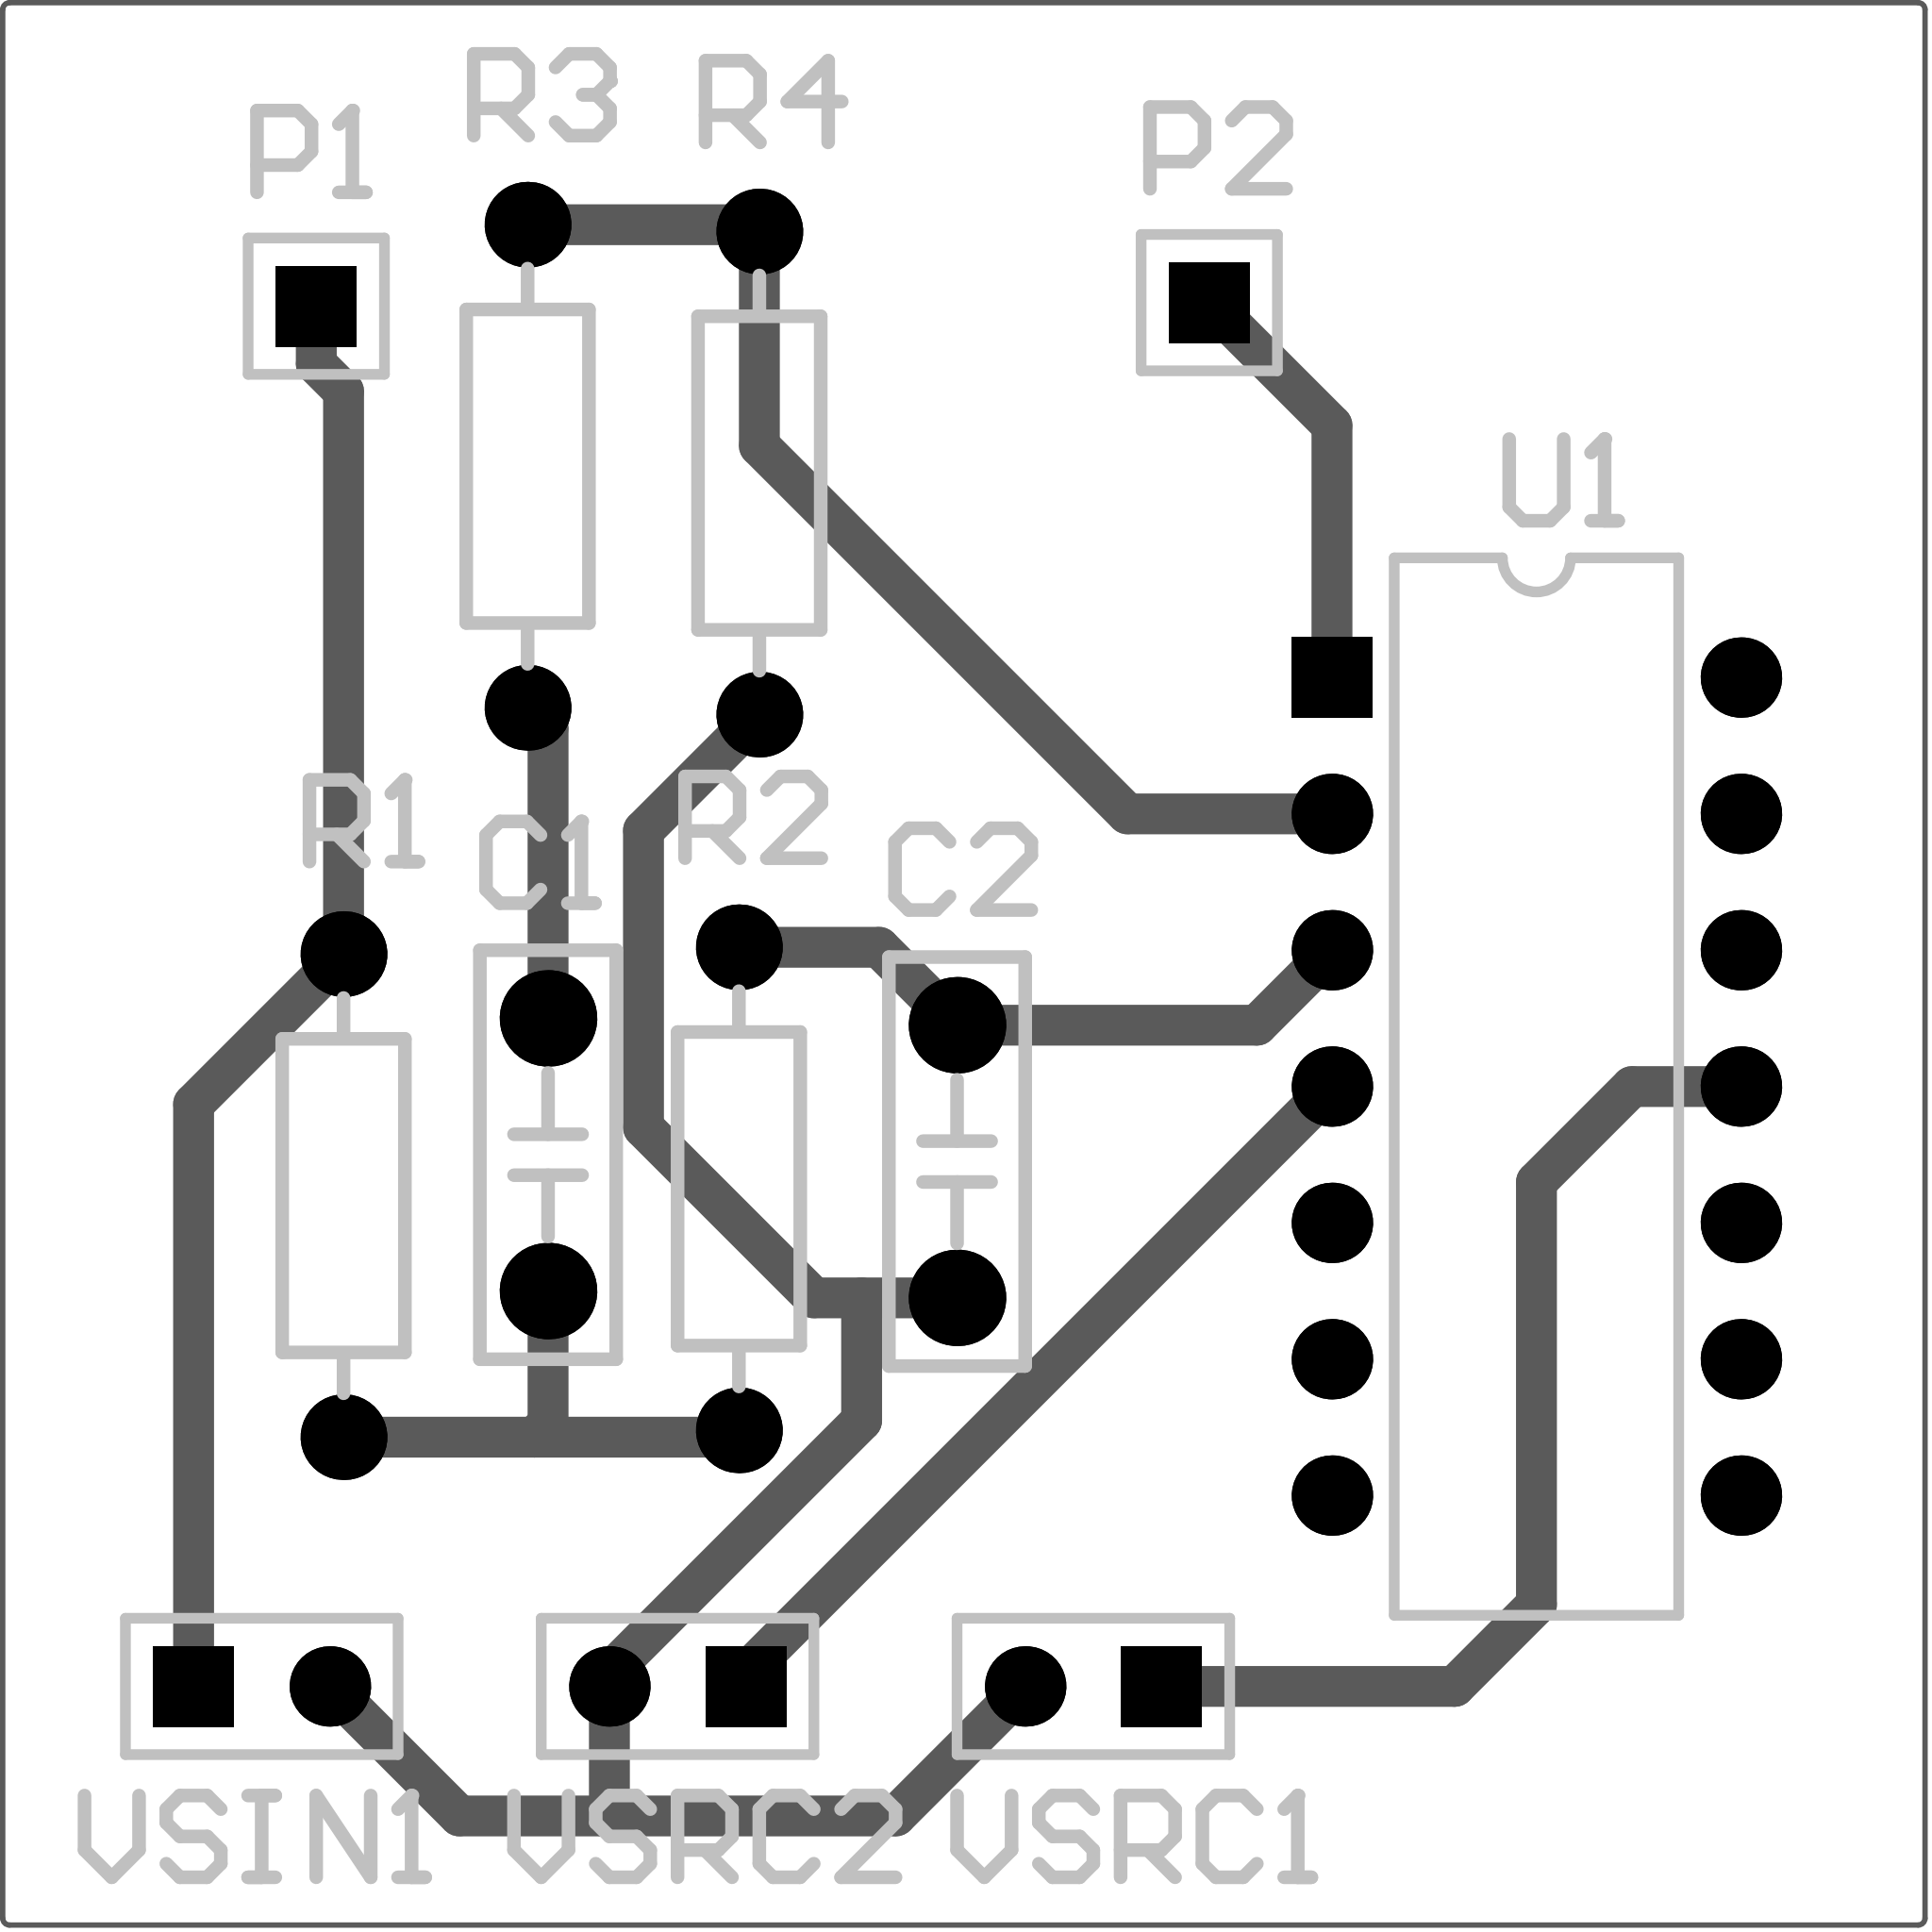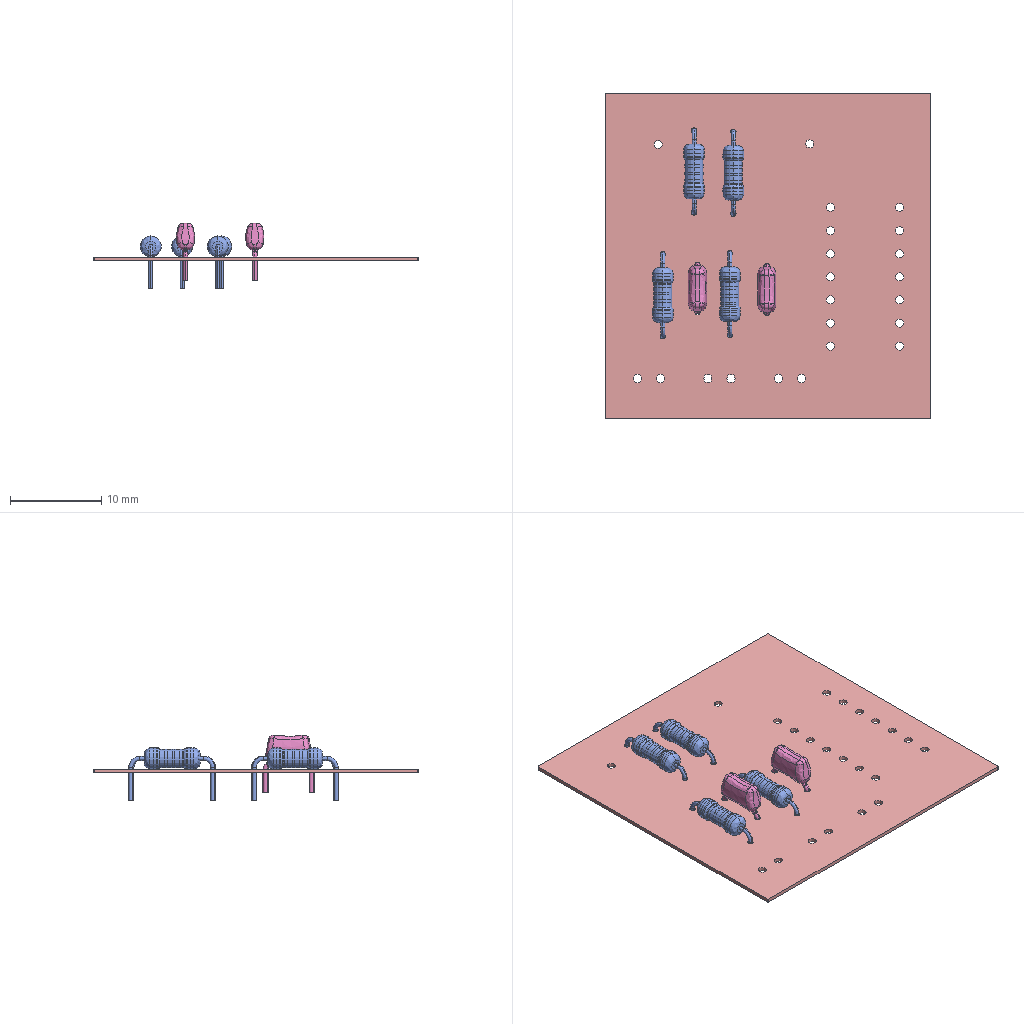Circuit board layout | Altium Designer | box 35.8 x 35.8 x 7.2 mm
Layer stack:
# Altium Designer layer stack of  (unit mm; dielectric type: 0 none, 1 core, 2 prepreg, 3 surface material)
index,name,kind,layer,copper_thickness_mm,dielectric_type,dielectric_thickness_mm,dielectric_material,dielectric_constant
0,Top Paste,other,,,,,,
1,Top Overlay,other,,,,,,
2,Top Solder,dielectric,,,3,0.0102,Solder Resist,3.5
3,Top Layer,copper,Top Layer,0.0356,,,,
4,Dielectric 1,dielectric,,,0,0.32,FR-4,4.8
5,Bottom Layer,copper,Bottom Layer,0.0356,,,,
6,Bottom Solder,dielectric,,,3,0.0102,Solder Resist,3.5
7,Bottom Overlay,other,,,,,,
8,Bottom Paste,other,,,,,,
# drill layer pairs: low layer,high layer
drill_pair,Top Layer,Bottom Layer
Part placement:
Designator,Comment,Layer,Footprint,Center-X(mm),Center-Y(mm),Rotation
VSRC2,12Vpos,TopLayer,HDR1X2,70.231,53.848,180
VSRC1,12Vneg,TopLayer,HDR1X2,77.978,53.848,180
VSIN1,1000HZ,TopLayer,HDR1X2,62.484,53.848,360
U1,LM324N,TopLayer,646-06,86.233,65.024,270
R4,3.184K,TopLayer,RS_1/4W,71.755,76.454,90
R3,3.184K,TopLayer,RS_1/4W,67.437,76.581,90
R2,796,TopLayer,RS_1/4W,71.374,63.119,90
R1,796,TopLayer,RS_1/4W,64.008,62.992,270
P2,HDR1X1,TopLayer,HDR1X1,80.137,79.629,0
P1,HDR1X1,TopLayer,HDR1X1,63.5,79.563,0
C2,0.1UF,TopLayer,MLCC5.08-A,75.438,63.627,90
C1,0.1UF,TopLayer,MLCC5.08-A,67.818,63.754,90
Pad and via stacks:
# Altium Designer via and pad stacks of  (unit mm). Each distinct definition once, with the count of objects using it.
# via: kind,start_layer,end_layer,hole_mm,diameter_mm,mode(0 simple;1 top-mid-bottom;2 full stack),diameter_per_layer,count,example_net
# pad: kind,layer,hole_mm,hole_type(0 round;1 square;2 slot),plating,top_size,top_shape(1 round;2 rect;3 octagon;9 rounded rect),mid_size,bottom_size,mode,footprint,size_per_layer,count,example
pad,Multi-Layer,0.9,0,plated,1.5x1.5,2,1.5x1.5,1.5x1.5,0,HDR1X2,,3,VSRC1.1
pad,Multi-Layer,0.9,0,plated,1.5x1.5,1,1.5x1.5,1.5x1.5,0,HDR1X2,,3,VSRC1.2
pad,Multi-Layer,0.7,0,plated,1.8x1.8,1,1.8x1.8,1.8x1.8,0,MLCC5.08-A,,4,C1.2
pad,Multi-Layer,0.9,0,plated,1.5x1.5,1,1.5x1.5,1.5x1.5,0,646-06,,13,U1.8
pad,Multi-Layer,0.9,0,plated,1.5x1.5,2,1.5x1.5,1.5x1.5,0,646-06,,1,U1.1
pad,Multi-Layer,0.9,2,plated,1.5x1.5,2,1.5x1.5,1.5x1.5,0,HDR1X1,,2,P1.1
pad,Multi-Layer,0.6,0,plated,1.6x1.6,1,1.6x1.6,1.6x1.6,0,RS 1/4W,,8,R2.2
Design rules, without the lines most boards share:
# Altium Designer design rules of  (exported by Altium Designer, unit mm)
# columns: name | kind | enabled | priority | scope1 | scope2 | descriptor | typed fields (field=value)
SilkToSilkClearance | 55 | enabled | 1 | All | All | Silk to Silk (Clearance=0mil) (All),(All) |
SilkToSolderMaskClearance | 54 | enabled | 1 | IsPad | All | Silk To Solder Mask (Clearance=0mil) (IsPad),(All) |
MinimumSolderMaskSliver | 53 | enabled | 1 | All | All | Minimum Solder Mask Sliver (Gap=0mil) (All),(All) |
HoleToHoleClearance | 52 | enabled | 1 | All | All | Hole To Hole Clearance (Gap=10mil) (All),(All) | gap=0.254
DiffPairsRouting | 51 | enabled | 1 | All | All | Differential Pairs Uncoupled Length using the Gap Constraints (Min=10mil) (Max=10mil) (Prefered=10mil)  and Width Constraints (Min=15mil) (Max=15mil) (Prefered=15mil) (All) |
SolderMaskExpansion | 13 | enabled | 1 | All | All | Solder Mask Expansion (Expansion =4mil) (All) | expansion=0.1016
PasteMaskExpansion | 14 | enabled | 1 | All | All | Paste Mask Expansion (Expansion =0mil) (All) | expansion=0
RoutingVias | 11 | enabled | 1 | All | All | Routing Via (MinHoleWidth=28mil) (MaxHoleWidth=28mil) (PreferredHoleWidth=28mil) (MinWidth=50mil) (MaxWidth=50mil) (PreferedWidth=50mil) (All) | via_min_hole=0.7112 via_max_hole=0.7112 via_preferred_diameter=1.27 via_preferred_hole=0.7112
Width | 2 | enabled | 1 | All | All | Width Constraint (Min=10mil) (Max=30mil) (Preferred=10mil) (All) |
PolygonConnect | 20 | enabled | 1 | All | All | Polygon Connect Rule(Relief Connect )(Conductor Width=10mil) (Relief Angle=90 Angle) (Entries=4) (Air Gap Width=10mil) (All),(All) | connect_style(0=relief,1=direct,2=none)=0 relief_conductor_width=0.254 relief_entries=4
PlaneConnect | 6 | enabled | 1 | All | All | Power Plane Connect Rule(Relief Connect )(Expansion=20mil) (Conductor Width=10mil) (Air Gap=10mil) (Entries=4) (All) | relief_conductor_width=0.254 relief_entries=4 relief_expansion=0.508
Clearance | 0 | enabled | 1 | All | All | Clearance Constraint (Gap=10mil) (All),(All) | gap=0.254
Classes set for this board:
# Altium Designer classes of  (member kind: 0 net, 1 component, 2 from-to, 3 pad, 4 layer, 5 differential pair, 6 design channel, 7 polygon, 8 structure, 9 xSignal)
# columns: class name | member kind | superclass | members
Sheet2 | 1 | no | C1; C2; P1; P2; R1; R2; R3; R4; U1; VSIN1; VSRC1; VSRC2;